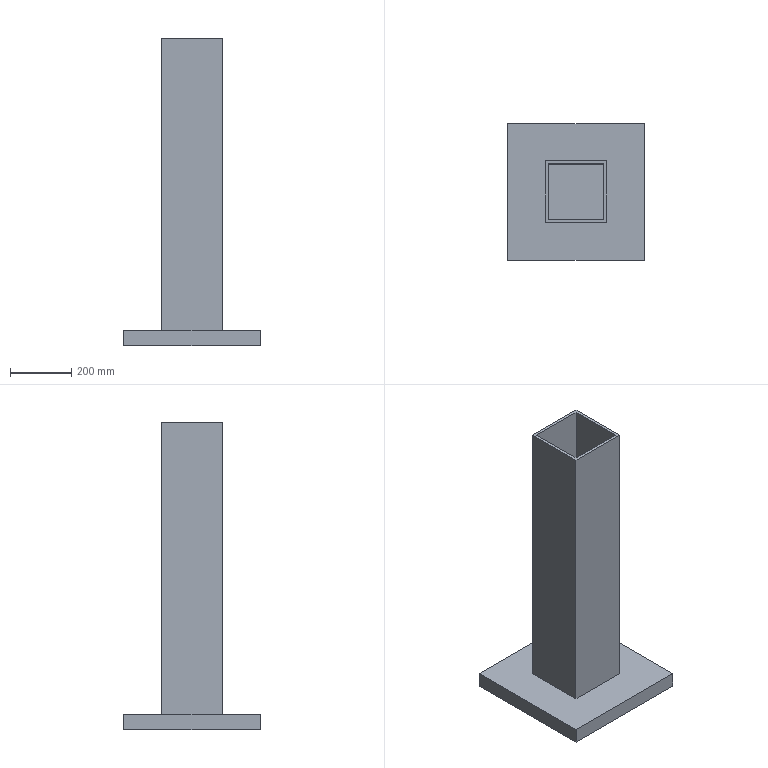Part | SolidWorks | features Extrusion 1, ICE 1 | 1 solid | 16 faces | box 445 x 445 x 1000 mm | volume 17121250 mm3 | plane 16
STEP:
#1=CARTESIAN_POINT('',(222.5,-222.5,50.));
#2=VERTEX_POINT('',#1);
#3=CARTESIAN_POINT('',(222.5,222.5,50.));
#4=VERTEX_POINT('',#3);
#5=CARTESIAN_POINT('',(222.5,222.5,50.));
#6=DIRECTION('',(0.,1.,0.));
#7=VECTOR('',#6,1000.);
#8=LINE('',#5,#7);
#9=EDGE_CURVE('',#2,#4,#8,.T.);
#10=ORIENTED_EDGE('',*,*,#9,.T.);
#11=CARTESIAN_POINT('',(-222.5,222.5,50.));
#12=VERTEX_POINT('',#11);
#13=CARTESIAN_POINT('',(-222.5,222.5,50.));
#14=DIRECTION('',(-1.,0.,0.));
#15=VECTOR('',#14,1000.);
#16=LINE('',#13,#15);
#17=EDGE_CURVE('',#4,#12,#16,.T.);
#18=ORIENTED_EDGE('',*,*,#17,.T.);
#19=CARTESIAN_POINT('',(-222.5,-222.5,50.));
#20=VERTEX_POINT('',#19);
#21=CARTESIAN_POINT('',(-222.5,222.5,50.));
#22=DIRECTION('',(0.,-1.,0.));
#23=VECTOR('',#22,1000.);
#24=LINE('',#21,#23);
#25=EDGE_CURVE('',#12,#20,#24,.T.);
#26=ORIENTED_EDGE('',*,*,#25,.T.);
#27=CARTESIAN_POINT('',(-222.5,-222.5,50.));
#28=DIRECTION('',(1.,0.,0.));
#29=VECTOR('',#28,1000.);
#30=LINE('',#27,#29);
#31=EDGE_CURVE('',#20,#2,#30,.T.);
#32=ORIENTED_EDGE('',*,*,#31,.T.);
#33=EDGE_LOOP('',(#10,#18,#26,#32));
#34=FACE_OUTER_BOUND('',#33,.T.);
#35=CARTESIAN_POINT('',(100.,100.,50.));
#36=VERTEX_POINT('',#35);
#37=CARTESIAN_POINT('',(-100.,100.,50.));
#38=VERTEX_POINT('',#37);
#39=CARTESIAN_POINT('',(-100.,100.,50.));
#40=DIRECTION('',(-1.,0.,0.));
#41=VECTOR('',#40,1000.);
#42=LINE('',#39,#41);
#43=EDGE_CURVE('',#36,#38,#42,.T.);
#44=ORIENTED_EDGE('',*,*,#43,.F.);
#45=CARTESIAN_POINT('',(100.,-100.,50.));
#46=VERTEX_POINT('',#45);
#47=CARTESIAN_POINT('',(100.,100.,50.));
#48=DIRECTION('',(0.,1.,0.));
#49=VECTOR('',#48,1000.);
#50=LINE('',#47,#49);
#51=EDGE_CURVE('',#46,#36,#50,.T.);
#52=ORIENTED_EDGE('',*,*,#51,.F.);
#53=CARTESIAN_POINT('',(-100.,-100.,50.));
#54=VERTEX_POINT('',#53);
#55=CARTESIAN_POINT('',(-100.,-100.,50.));
#56=DIRECTION('',(1.,0.,0.));
#57=VECTOR('',#56,1000.);
#58=LINE('',#55,#57);
#59=EDGE_CURVE('',#54,#46,#58,.T.);
#60=ORIENTED_EDGE('',*,*,#59,.F.);
#61=CARTESIAN_POINT('',(-100.,100.,50.));
#62=DIRECTION('',(0.,-1.,0.));
#63=VECTOR('',#62,1000.);
#64=LINE('',#61,#63);
#65=EDGE_CURVE('',#38,#54,#64,.T.);
#66=ORIENTED_EDGE('',*,*,#65,.F.);
#67=EDGE_LOOP('',(#44,#52,#60,#66));
#68=FACE_BOUND('',#67,.T.);
#69=CARTESIAN_POINT('',(0.,0.,50.));
#70=DIRECTION('',(0.,0.,1.));
#71=DIRECTION('',(1.,0.,0.));
#72=AXIS2_PLACEMENT_3D('',#69,#70,#71);
#73=PLANE('',#72);
#74=ADVANCED_FACE('',(#34,#68),#73,.T.);
#75=CARTESIAN_POINT('',(222.5,-222.5,0.));
#76=VERTEX_POINT('',#75);
#77=CARTESIAN_POINT('',(222.5,222.5,0.));
#78=VERTEX_POINT('',#77);
#79=CARTESIAN_POINT('',(222.5,222.5,0.));
#80=DIRECTION('',(0.,1.,0.));
#81=VECTOR('',#80,1000.);
#82=LINE('',#79,#81);
#83=EDGE_CURVE('',#76,#78,#82,.T.);
#84=ORIENTED_EDGE('',*,*,#83,.T.);
#85=CARTESIAN_POINT('',(222.5,222.5,50.));
#86=DIRECTION('',(0.,0.,-1.));
#87=VECTOR('',#86,1000.);
#88=LINE('',#85,#87);
#89=EDGE_CURVE('',#4,#78,#88,.T.);
#90=ORIENTED_EDGE('',*,*,#89,.F.);
#91=ORIENTED_EDGE('',*,*,#9,.F.);
#92=CARTESIAN_POINT('',(222.5,-222.5,50.));
#93=DIRECTION('',(0.,0.,-1.));
#94=VECTOR('',#93,1000.);
#95=LINE('',#92,#94);
#96=EDGE_CURVE('',#2,#76,#95,.T.);
#97=ORIENTED_EDGE('',*,*,#96,.T.);
#98=EDGE_LOOP('',(#84,#90,#91,#97));
#99=FACE_OUTER_BOUND('',#98,.T.);
#100=CARTESIAN_POINT('',(222.5,222.5,50.));
#101=DIRECTION('',(-1.,0.,0.));
#102=DIRECTION('',(0.,-1.,0.));
#103=AXIS2_PLACEMENT_3D('',#100,#101,#102);
#104=PLANE('',#103);
#105=ADVANCED_FACE('',(#99),#104,.F.);
#106=CARTESIAN_POINT('',(-222.5,222.5,0.));
#107=VERTEX_POINT('',#106);
#108=CARTESIAN_POINT('',(-222.5,222.5,0.));
#109=DIRECTION('',(-1.,0.,0.));
#110=VECTOR('',#109,1000.);
#111=LINE('',#108,#110);
#112=EDGE_CURVE('',#78,#107,#111,.T.);
#113=ORIENTED_EDGE('',*,*,#112,.T.);
#114=CARTESIAN_POINT('',(-222.5,222.5,50.));
#115=DIRECTION('',(0.,0.,-1.));
#116=VECTOR('',#115,1000.);
#117=LINE('',#114,#116);
#118=EDGE_CURVE('',#12,#107,#117,.T.);
#119=ORIENTED_EDGE('',*,*,#118,.F.);
#120=ORIENTED_EDGE('',*,*,#17,.F.);
#121=ORIENTED_EDGE('',*,*,#89,.T.);
#122=EDGE_LOOP('',(#113,#119,#120,#121));
#123=FACE_OUTER_BOUND('',#122,.T.);
#124=CARTESIAN_POINT('',(-222.5,222.5,50.));
#125=DIRECTION('',(0.,-1.,0.));
#126=DIRECTION('',(0.,0.,-1.));
#127=AXIS2_PLACEMENT_3D('',#124,#125,#126);
#128=PLANE('',#127);
#129=ADVANCED_FACE('',(#123),#128,.F.);
#130=CARTESIAN_POINT('',(-222.5,-222.5,0.));
#131=VERTEX_POINT('',#130);
#132=CARTESIAN_POINT('',(-222.5,222.5,0.));
#133=DIRECTION('',(0.,-1.,0.));
#134=VECTOR('',#133,1000.);
#135=LINE('',#132,#134);
#136=EDGE_CURVE('',#107,#131,#135,.T.);
#137=ORIENTED_EDGE('',*,*,#136,.T.);
#138=CARTESIAN_POINT('',(-222.5,-222.5,50.));
#139=DIRECTION('',(0.,0.,-1.));
#140=VECTOR('',#139,1000.);
#141=LINE('',#138,#140);
#142=EDGE_CURVE('',#20,#131,#141,.T.);
#143=ORIENTED_EDGE('',*,*,#142,.F.);
#144=ORIENTED_EDGE('',*,*,#25,.F.);
#145=ORIENTED_EDGE('',*,*,#118,.T.);
#146=EDGE_LOOP('',(#137,#143,#144,#145));
#147=FACE_OUTER_BOUND('',#146,.T.);
#148=CARTESIAN_POINT('',(-222.5,222.5,50.));
#149=DIRECTION('',(1.,0.,0.));
#150=DIRECTION('',(0.,1.,0.));
#151=AXIS2_PLACEMENT_3D('',#148,#149,#150);
#152=PLANE('',#151);
#153=ADVANCED_FACE('',(#147),#152,.F.);
#154=CARTESIAN_POINT('',(-222.5,-222.5,0.));
#155=DIRECTION('',(1.,0.,0.));
#156=VECTOR('',#155,1000.);
#157=LINE('',#154,#156);
#158=EDGE_CURVE('',#131,#76,#157,.T.);
#159=ORIENTED_EDGE('',*,*,#158,.T.);
#160=ORIENTED_EDGE('',*,*,#96,.F.);
#161=ORIENTED_EDGE('',*,*,#31,.F.);
#162=ORIENTED_EDGE('',*,*,#142,.T.);
#163=EDGE_LOOP('',(#159,#160,#161,#162));
#164=FACE_OUTER_BOUND('',#163,.T.);
#165=CARTESIAN_POINT('',(-222.5,-222.5,50.));
#166=DIRECTION('',(0.,1.,0.));
#167=DIRECTION('',(0.,0.,1.));
#168=AXIS2_PLACEMENT_3D('',#165,#166,#167);
#169=PLANE('',#168);
#170=ADVANCED_FACE('',(#164),#169,.F.);
#171=ORIENTED_EDGE('',*,*,#83,.F.);
#172=ORIENTED_EDGE('',*,*,#158,.F.);
#173=ORIENTED_EDGE('',*,*,#136,.F.);
#174=ORIENTED_EDGE('',*,*,#112,.F.);
#175=EDGE_LOOP('',(#171,#172,#173,#174));
#176=FACE_OUTER_BOUND('',#175,.T.);
#177=CARTESIAN_POINT('',(0.,0.,0.));
#178=DIRECTION('',(0.,0.,1.));
#179=DIRECTION('',(1.,0.,0.));
#180=AXIS2_PLACEMENT_3D('',#177,#178,#179);
#181=PLANE('',#180);
#182=ADVANCED_FACE('',(#176),#181,.F.);
#183=CARTESIAN_POINT('',(100.,-100.,1000.));
#184=VERTEX_POINT('',#183);
#185=CARTESIAN_POINT('',(100.,100.,1000.));
#186=VERTEX_POINT('',#185);
#187=CARTESIAN_POINT('',(100.,100.,1000.));
#188=DIRECTION('',(0.,1.,0.));
#189=VECTOR('',#188,1000.);
#190=LINE('',#187,#189);
#191=EDGE_CURVE('',#184,#186,#190,.T.);
#192=ORIENTED_EDGE('',*,*,#191,.T.);
#193=CARTESIAN_POINT('',(-100.,100.,1000.));
#194=VERTEX_POINT('',#193);
#195=CARTESIAN_POINT('',(-100.,100.,1000.));
#196=DIRECTION('',(-1.,0.,0.));
#197=VECTOR('',#196,1000.);
#198=LINE('',#195,#197);
#199=EDGE_CURVE('',#186,#194,#198,.T.);
#200=ORIENTED_EDGE('',*,*,#199,.T.);
#201=CARTESIAN_POINT('',(-100.,-100.,1000.));
#202=VERTEX_POINT('',#201);
#203=CARTESIAN_POINT('',(-100.,100.,1000.));
#204=DIRECTION('',(0.,-1.,0.));
#205=VECTOR('',#204,1000.);
#206=LINE('',#203,#205);
#207=EDGE_CURVE('',#194,#202,#206,.T.);
#208=ORIENTED_EDGE('',*,*,#207,.T.);
#209=CARTESIAN_POINT('',(-100.,-100.,1000.));
#210=DIRECTION('',(1.,0.,0.));
#211=VECTOR('',#210,1000.);
#212=LINE('',#209,#211);
#213=EDGE_CURVE('',#202,#184,#212,.T.);
#214=ORIENTED_EDGE('',*,*,#213,.T.);
#215=EDGE_LOOP('',(#192,#200,#208,#214));
#216=FACE_OUTER_BOUND('',#215,.T.);
#217=CARTESIAN_POINT('',(90.,90.,1000.));
#218=VERTEX_POINT('',#217);
#219=CARTESIAN_POINT('',(-90.,90.,1000.));
#220=VERTEX_POINT('',#219);
#221=CARTESIAN_POINT('',(-90.,90.,1000.));
#222=DIRECTION('',(-1.,0.,0.));
#223=VECTOR('',#222,1000.);
#224=LINE('',#221,#223);
#225=EDGE_CURVE('',#218,#220,#224,.T.);
#226=ORIENTED_EDGE('',*,*,#225,.F.);
#227=CARTESIAN_POINT('',(90.,-90.,1000.));
#228=VERTEX_POINT('',#227);
#229=CARTESIAN_POINT('',(90.,90.,1000.));
#230=DIRECTION('',(0.,1.,0.));
#231=VECTOR('',#230,1000.);
#232=LINE('',#229,#231);
#233=EDGE_CURVE('',#228,#218,#232,.T.);
#234=ORIENTED_EDGE('',*,*,#233,.F.);
#235=CARTESIAN_POINT('',(-90.,-90.,1000.));
#236=VERTEX_POINT('',#235);
#237=CARTESIAN_POINT('',(-90.,-90.,1000.));
#238=DIRECTION('',(1.,0.,0.));
#239=VECTOR('',#238,1000.);
#240=LINE('',#237,#239);
#241=EDGE_CURVE('',#236,#228,#240,.T.);
#242=ORIENTED_EDGE('',*,*,#241,.F.);
#243=CARTESIAN_POINT('',(-90.,90.,1000.));
#244=DIRECTION('',(0.,-1.,0.));
#245=VECTOR('',#244,1000.);
#246=LINE('',#243,#245);
#247=EDGE_CURVE('',#220,#236,#246,.T.);
#248=ORIENTED_EDGE('',*,*,#247,.F.);
#249=EDGE_LOOP('',(#226,#234,#242,#248));
#250=FACE_BOUND('',#249,.T.);
#251=CARTESIAN_POINT('',(0.,0.,1000.));
#252=DIRECTION('',(0.,0.,1.));
#253=DIRECTION('',(1.,0.,0.));
#254=AXIS2_PLACEMENT_3D('',#251,#252,#253);
#255=PLANE('',#254);
#256=ADVANCED_FACE('',(#216,#250),#255,.T.);
#257=ORIENTED_EDGE('',*,*,#51,.T.);
#258=CARTESIAN_POINT('',(100.,100.,1000.));
#259=DIRECTION('',(0.,0.,-1.));
#260=VECTOR('',#259,1000.);
#261=LINE('',#258,#260);
#262=EDGE_CURVE('',#186,#36,#261,.T.);
#263=ORIENTED_EDGE('',*,*,#262,.F.);
#264=ORIENTED_EDGE('',*,*,#191,.F.);
#265=CARTESIAN_POINT('',(100.,-100.,1000.));
#266=DIRECTION('',(0.,0.,-1.));
#267=VECTOR('',#266,1000.);
#268=LINE('',#265,#267);
#269=EDGE_CURVE('',#184,#46,#268,.T.);
#270=ORIENTED_EDGE('',*,*,#269,.T.);
#271=EDGE_LOOP('',(#257,#263,#264,#270));
#272=FACE_OUTER_BOUND('',#271,.T.);
#273=CARTESIAN_POINT('',(100.,100.,1000.));
#274=DIRECTION('',(-1.,0.,0.));
#275=DIRECTION('',(0.,-1.,0.));
#276=AXIS2_PLACEMENT_3D('',#273,#274,#275);
#277=PLANE('',#276);
#278=ADVANCED_FACE('',(#272),#277,.F.);
#279=ORIENTED_EDGE('',*,*,#43,.T.);
#280=CARTESIAN_POINT('',(-100.,100.,1000.));
#281=DIRECTION('',(0.,0.,-1.));
#282=VECTOR('',#281,1000.);
#283=LINE('',#280,#282);
#284=EDGE_CURVE('',#194,#38,#283,.T.);
#285=ORIENTED_EDGE('',*,*,#284,.F.);
#286=ORIENTED_EDGE('',*,*,#199,.F.);
#287=ORIENTED_EDGE('',*,*,#262,.T.);
#288=EDGE_LOOP('',(#279,#285,#286,#287));
#289=FACE_OUTER_BOUND('',#288,.T.);
#290=CARTESIAN_POINT('',(-100.,100.,1000.));
#291=DIRECTION('',(0.,-1.,0.));
#292=DIRECTION('',(0.,0.,-1.));
#293=AXIS2_PLACEMENT_3D('',#290,#291,#292);
#294=PLANE('',#293);
#295=ADVANCED_FACE('',(#289),#294,.F.);
#296=ORIENTED_EDGE('',*,*,#65,.T.);
#297=CARTESIAN_POINT('',(-100.,-100.,1000.));
#298=DIRECTION('',(0.,0.,-1.));
#299=VECTOR('',#298,1000.);
#300=LINE('',#297,#299);
#301=EDGE_CURVE('',#202,#54,#300,.T.);
#302=ORIENTED_EDGE('',*,*,#301,.F.);
#303=ORIENTED_EDGE('',*,*,#207,.F.);
#304=ORIENTED_EDGE('',*,*,#284,.T.);
#305=EDGE_LOOP('',(#296,#302,#303,#304));
#306=FACE_OUTER_BOUND('',#305,.T.);
#307=CARTESIAN_POINT('',(-100.,100.,1000.));
#308=DIRECTION('',(1.,0.,0.));
#309=DIRECTION('',(0.,1.,0.));
#310=AXIS2_PLACEMENT_3D('',#307,#308,#309);
#311=PLANE('',#310);
#312=ADVANCED_FACE('',(#306),#311,.F.);
#313=ORIENTED_EDGE('',*,*,#59,.T.);
#314=ORIENTED_EDGE('',*,*,#269,.F.);
#315=ORIENTED_EDGE('',*,*,#213,.F.);
#316=ORIENTED_EDGE('',*,*,#301,.T.);
#317=EDGE_LOOP('',(#313,#314,#315,#316));
#318=FACE_OUTER_BOUND('',#317,.T.);
#319=CARTESIAN_POINT('',(-100.,-100.,1000.));
#320=DIRECTION('',(0.,1.,0.));
#321=DIRECTION('',(0.,0.,1.));
#322=AXIS2_PLACEMENT_3D('',#319,#320,#321);
#323=PLANE('',#322);
#324=ADVANCED_FACE('',(#318),#323,.F.);
#325=CARTESIAN_POINT('',(90.,-90.,50.));
#326=VERTEX_POINT('',#325);
#327=CARTESIAN_POINT('',(90.,90.,50.));
#328=VERTEX_POINT('',#327);
#329=CARTESIAN_POINT('',(90.,90.,50.));
#330=DIRECTION('',(0.,1.,0.));
#331=VECTOR('',#330,1000.);
#332=LINE('',#329,#331);
#333=EDGE_CURVE('',#326,#328,#332,.T.);
#334=ORIENTED_EDGE('',*,*,#333,.F.);
#335=CARTESIAN_POINT('',(90.,-90.,1000.));
#336=DIRECTION('',(0.,0.,-1.));
#337=VECTOR('',#336,1000.);
#338=LINE('',#335,#337);
#339=EDGE_CURVE('',#228,#326,#338,.T.);
#340=ORIENTED_EDGE('',*,*,#339,.F.);
#341=ORIENTED_EDGE('',*,*,#233,.T.);
#342=CARTESIAN_POINT('',(90.,90.,1000.));
#343=DIRECTION('',(0.,0.,-1.));
#344=VECTOR('',#343,1000.);
#345=LINE('',#342,#344);
#346=EDGE_CURVE('',#218,#328,#345,.T.);
#347=ORIENTED_EDGE('',*,*,#346,.T.);
#348=EDGE_LOOP('',(#334,#340,#341,#347));
#349=FACE_OUTER_BOUND('',#348,.T.);
#350=CARTESIAN_POINT('',(90.,90.,1000.));
#351=DIRECTION('',(-1.,0.,0.));
#352=DIRECTION('',(0.,-1.,0.));
#353=AXIS2_PLACEMENT_3D('',#350,#351,#352);
#354=PLANE('',#353);
#355=ADVANCED_FACE('',(#349),#354,.T.);
#356=CARTESIAN_POINT('',(-90.,90.,50.));
#357=VERTEX_POINT('',#356);
#358=CARTESIAN_POINT('',(-90.,90.,50.));
#359=DIRECTION('',(-1.,0.,0.));
#360=VECTOR('',#359,1000.);
#361=LINE('',#358,#360);
#362=EDGE_CURVE('',#328,#357,#361,.T.);
#363=ORIENTED_EDGE('',*,*,#362,.F.);
#364=ORIENTED_EDGE('',*,*,#346,.F.);
#365=ORIENTED_EDGE('',*,*,#225,.T.);
#366=CARTESIAN_POINT('',(-90.,90.,1000.));
#367=DIRECTION('',(0.,0.,-1.));
#368=VECTOR('',#367,1000.);
#369=LINE('',#366,#368);
#370=EDGE_CURVE('',#220,#357,#369,.T.);
#371=ORIENTED_EDGE('',*,*,#370,.T.);
#372=EDGE_LOOP('',(#363,#364,#365,#371));
#373=FACE_OUTER_BOUND('',#372,.T.);
#374=CARTESIAN_POINT('',(-90.,90.,1000.));
#375=DIRECTION('',(0.,-1.,0.));
#376=DIRECTION('',(0.,0.,-1.));
#377=AXIS2_PLACEMENT_3D('',#374,#375,#376);
#378=PLANE('',#377);
#379=ADVANCED_FACE('',(#373),#378,.T.);
#380=CARTESIAN_POINT('',(-90.,-90.,50.));
#381=VERTEX_POINT('',#380);
#382=CARTESIAN_POINT('',(-90.,90.,50.));
#383=DIRECTION('',(0.,-1.,0.));
#384=VECTOR('',#383,1000.);
#385=LINE('',#382,#384);
#386=EDGE_CURVE('',#357,#381,#385,.T.);
#387=ORIENTED_EDGE('',*,*,#386,.F.);
#388=ORIENTED_EDGE('',*,*,#370,.F.);
#389=ORIENTED_EDGE('',*,*,#247,.T.);
#390=CARTESIAN_POINT('',(-90.,-90.,1000.));
#391=DIRECTION('',(0.,0.,-1.));
#392=VECTOR('',#391,1000.);
#393=LINE('',#390,#392);
#394=EDGE_CURVE('',#236,#381,#393,.T.);
#395=ORIENTED_EDGE('',*,*,#394,.T.);
#396=EDGE_LOOP('',(#387,#388,#389,#395));
#397=FACE_OUTER_BOUND('',#396,.T.);
#398=CARTESIAN_POINT('',(-90.,90.,1000.));
#399=DIRECTION('',(1.,0.,0.));
#400=DIRECTION('',(0.,1.,0.));
#401=AXIS2_PLACEMENT_3D('',#398,#399,#400);
#402=PLANE('',#401);
#403=ADVANCED_FACE('',(#397),#402,.T.);
#404=CARTESIAN_POINT('',(-90.,-90.,50.));
#405=DIRECTION('',(1.,0.,0.));
#406=VECTOR('',#405,1000.);
#407=LINE('',#404,#406);
#408=EDGE_CURVE('',#381,#326,#407,.T.);
#409=ORIENTED_EDGE('',*,*,#408,.F.);
#410=ORIENTED_EDGE('',*,*,#394,.F.);
#411=ORIENTED_EDGE('',*,*,#241,.T.);
#412=ORIENTED_EDGE('',*,*,#339,.T.);
#413=EDGE_LOOP('',(#409,#410,#411,#412));
#414=FACE_OUTER_BOUND('',#413,.T.);
#415=CARTESIAN_POINT('',(-90.,-90.,1000.));
#416=DIRECTION('',(0.,1.,0.));
#417=DIRECTION('',(0.,0.,1.));
#418=AXIS2_PLACEMENT_3D('',#415,#416,#417);
#419=PLANE('',#418);
#420=ADVANCED_FACE('',(#414),#419,.T.);
#421=ORIENTED_EDGE('',*,*,#333,.T.);
#422=ORIENTED_EDGE('',*,*,#362,.T.);
#423=ORIENTED_EDGE('',*,*,#386,.T.);
#424=ORIENTED_EDGE('',*,*,#408,.T.);
#425=EDGE_LOOP('',(#421,#422,#423,#424));
#426=FACE_OUTER_BOUND('',#425,.T.);
#427=CARTESIAN_POINT('',(0.,0.,50.));
#428=DIRECTION('',(0.,0.,1.));
#429=DIRECTION('',(1.,0.,0.));
#430=AXIS2_PLACEMENT_3D('',#427,#428,#429);
#431=PLANE('',#430);
#432=ADVANCED_FACE('',(#426),#431,.T.);
#433=CLOSED_SHELL('',(#74,#105,#129,#153,#170,#182,#256,#278,#295,#312,#324,#355,#379,#403,#420,#432));
#434=MANIFOLD_SOLID_BREP('',#433);
#435=CARTESIAN_POINT('',(0.,0.,0.));
#436=DIRECTION('',(0.,0.,1.));
#437=DIRECTION('',(1.,0.,0.));
#438=AXIS2_PLACEMENT_3D('',#435,#436,#437);
#439=(LENGTH_UNIT()NAMED_UNIT(*)SI_UNIT(.MILLI.,.METRE.));
#440=UNCERTAINTY_MEASURE_WITH_UNIT(LENGTH_MEASURE(0.00001),#439,'','');
#441=(NAMED_UNIT(*)PLANE_ANGLE_UNIT()SI_UNIT($,.RADIAN.));
#442=(NAMED_UNIT(*)SI_UNIT($,.STERADIAN.)SOLID_ANGLE_UNIT());
#443=(GEOMETRIC_REPRESENTATION_CONTEXT(3)GLOBAL_UNCERTAINTY_ASSIGNED_CONTEXT((#440))GLOBAL_UNIT_ASSIGNED_CONTEXT((#439,#441,#442))REPRESENTATION_CONTEXT('',''));
#444=ADVANCED_BREP_SHAPE_REPRESENTATION('',(#434,#438),#443);